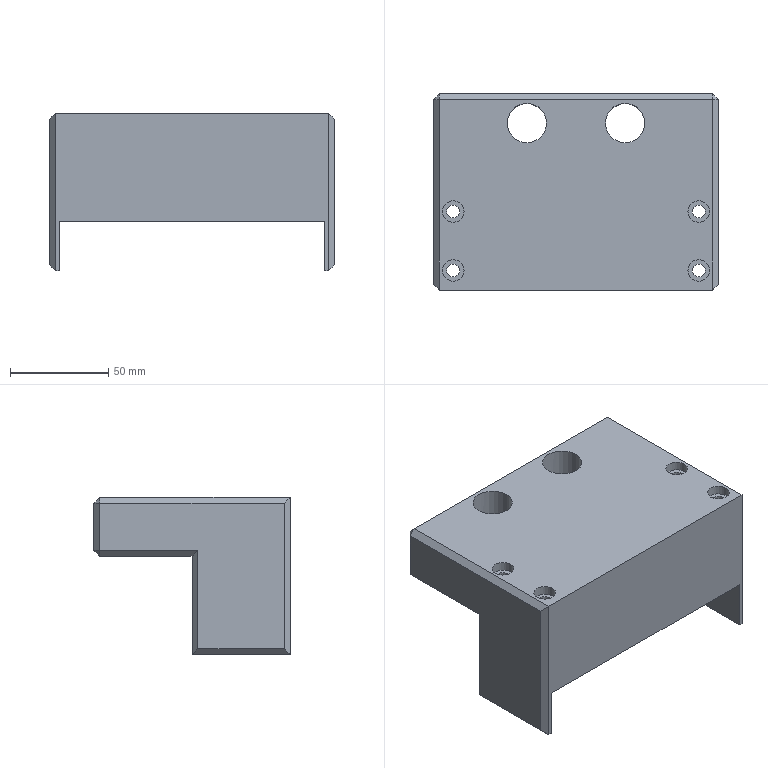NC program | NX | posted with a generic post | part box 145 x 100 x 80 mm
Whole program:
N10 G17 G21 G94 G90
(DRILLING_COPY_2 , TOOL : D8A45)
N12 T06 M6
N14 G54
N16 G17 G0 G90 X-62.5 Y-40. B0. C0. S3000 M3
N18 G43 Z30. H6
N20 G94 G81 G98 Z-1. F150. R3.
N22 Y-10.
N24 X-25. Y35.
N26 X25.
N28 X62.5 Y-10.
N30 Y-40.
N32 G80
N34 G0 X62.5 Y-40. Z30.
N36 M5
(DRILLING_COPY_COPY_COPY_COPY_1_COPY , TOOL : 6.6ZT)
N38 T15 M6
N40 G54
N42 G17 G0 G90 X-62.5 Y-10. B0. C0. S2000 M3
N44 G43 Z30. H15
N46 G94 G83 G98 Z-58.483 F150. Q2. R3.
N48 Y-40.
N50 X62.5
N52 Y-10.
N54 G80
N56 G0 X62.5 Y-10. Z30.
N58 M5
(DRILLING_COPY_COPY_COPY_COPY_1_COPY_COPY , TOOL : 10.5ZT)
N60 T17 M6
N62 G54
N64 G17 G0 G90 X-25. Y35. B0. C0. S1000 M3
N66 G43 Z30. H17
N68 G94 G83 G98 Z-34.655 F150. Q2. R3.
N70 X25.
N72 G80
N74 G0 X25. Y35. Z30.
N76 M5
(刀补12_COPY , TOOL : D10JING)
N78 T04 M6
N80 G54
N82 G17 G0 G90 X-25. Y35. B0. C0. S7000 M3
N84 G43 Z30. H4
N86 Z0.5
N88 G94 G3 X-22.55 Y32.55 R2.45 F1200.
N90 X-20.1 Y35. R2.45
N92 X-20.1 Y35. Z-0.5 I-4.9 J0.
N94 X-20.1 Y35. Z-1.5 I-4.9 J0.
N96 X-20.1 Y35. Z-2.5 I-4.9 J0.
N98 X-20.1 Y35. Z-3.5 I-4.9 J0.
N100 X-20.1 Y35. Z-4.5 I-4.9 J0.
N102 X-20.1 Y35. Z-5.5 I-4.9 J0.
N104 X-20.1 Y35. Z-6.5 I-4.9 J0.
N106 X-20.1 Y35. Z-7.5 I-4.9 J0.
N108 X-20.1 Y35. Z-8.5 I-4.9 J0.
N110 X-20.1 Y35. Z-9.5 I-4.9 J0.
N112 X-20.1 Y35. Z-10.5 I-4.9 J0.
N114 X-20.1 Y35. Z-11.5 I-4.9 J0.
N116 X-20.1 Y35. Z-12.5 I-4.9 J0.
N118 X-20.1 Y35. Z-13.5 I-4.9 J0.
N120 X-20.1 Y35. Z-14.5 I-4.9 J0.
N122 X-20.1 Y35. Z-15.5 I-4.9 J0.
N124 X-20.1 Y35. Z-16.5 I-4.9 J0.
N126 X-20.1 Y35. Z-17.5 I-4.9 J0.
N128 X-20.1 Y35. Z-18.5 I-4.9 J0.
N130 X-20.1 Y35. Z-19.5 I-4.9 J0.
N132 X-20.1 Y35. Z-20.5 I-4.9 J0.
N134 X-20.1 Y35. Z-21.5 I-4.9 J0.
N136 X-20.1 Y35. Z-22.5 I-4.9 J0.
N138 X-20.1 Y35. Z-23.5 I-4.9 J0.
N140 X-20.1 Y35. Z-24.5 I-4.9 J0.
N142 X-20.1 Y35. Z-25.5 I-4.9 J0.
N144 X-20.1 Y35. Z-26.5 I-4.9 J0.
N146 X-20.1 Y35. Z-27.5 I-4.9 J0.
N148 X-20.1 Y35. Z-28.5 I-4.9 J0.
N150 X-20.1 Y35. Z-29.5 I-4.9 J0.
N152 X-29.9 Y35. Z-30. I-4.9 J0.
N154 X-25. Y30.1 R4.9
N156 X-29.9 Y35. R-4.9
N158 X-27.45 Y32.55 R2.45
N160 X-25. Y35. R2.45
N162 G0 Z30.
N164 X25.
N166 Z0.5
N168 G3 X27.45 Y32.55 R2.45
N170 X29.9 Y35. R2.45
N172 X29.9 Y35. Z-0.5 I-4.9 J0.
N174 X29.9 Y35. Z-1.5 I-4.9 J0.
N176 X29.9 Y35. Z-2.5 I-4.9 J0.
N178 X29.9 Y35. Z-3.5 I-4.9 J0.
N180 X29.9 Y35. Z-4.5 I-4.9 J0.
N182 X29.9 Y35. Z-5.5 I-4.9 J0.
N184 X29.9 Y35. Z-6.5 I-4.9 J0.
N186 X29.9 Y35. Z-7.5 I-4.9 J0.
N188 X29.9 Y35. Z-8.5 I-4.9 J0.
N190 X29.9 Y35. Z-9.5 I-4.9 J0.
N192 X29.9 Y35. Z-10.5 I-4.9 J0.
N194 X29.9 Y35. Z-11.5 I-4.9 J0.
N196 X29.9 Y35. Z-12.5 I-4.9 J0.
N198 X29.9 Y35. Z-13.5 I-4.9 J0.
N200 X29.9 Y35. Z-14.5 I-4.9 J0.
N202 X29.9 Y35. Z-15.5 I-4.9 J0.
N204 X29.9 Y35. Z-16.5 I-4.9 J0.
N206 X29.9 Y35. Z-17.5 I-4.9 J0.
N208 X29.9 Y35. Z-18.5 I-4.9 J0.
N210 X29.9 Y35. Z-19.5 I-4.9 J0.
N212 X29.9 Y35. Z-20.5 I-4.9 J0.
N214 X29.9 Y35. Z-21.5 I-4.9 J0.
N216 X29.9 Y35. Z-22.5 I-4.9 J0.
N218 X29.9 Y35. Z-23.5 I-4.9 J0.
N220 X29.9 Y35. Z-24.5 I-4.9 J0.
N222 X29.9 Y35. Z-25.5 I-4.9 J0.
N224 X29.9 Y35. Z-26.5 I-4.9 J0.
N226 X29.9 Y35. Z-27.5 I-4.9 J0.
N228 X29.9 Y35. Z-28.5 I-4.9 J0.
N230 X29.9 Y35. Z-29.5 I-4.9 J0.
N232 X20.1 Y35. Z-30. I-4.9 J0.
N234 X25. Y30.1 R4.9
N236 X20.1 Y35. R-4.9
N238 X22.55 Y32.55 R2.45
N240 X25. Y35. R2.45
N242 G0 Z30.
N244 M5
(HOLE_MILLING , TOOL : D6)
N246 T02 M6
N248 G54
N250 G17 G0 G90 X-62.5 Y-10. B0. C0. S8000 M3
N252 G43 Z30. H2
N254 Z0.5
N256 G94 G3 X-61.25 Y-11.25 R1.25 F1000.
N258 X-60. Y-10. R1.25
N260 X-60. Y-10. Z0. I-2.5 J0.
N262 X-60. Y-10. Z-0.5 I-2.5 J0.
N264 X-60. Y-10. Z-1. I-2.5 J0.
N266 X-60. Y-10. Z-1.5 I-2.5 J0.
N268 X-60. Y-10. Z-2. I-2.5 J0.
N270 X-60. Y-10. Z-2.5 I-2.5 J0.
N272 X-60. Y-10. Z-3. I-2.5 J0.
N274 X-60. Y-10. Z-3.5 I-2.5 J0.
N276 X-60. Y-10. Z-4. I-2.5 J0.
N278 X-60. Y-10. Z-4.5 I-2.5 J0.
N280 X-64.523 Y-8.531 Z-4.7 R2.5
N282 X-63.969 Y-12.023 R2.5
N284 X-64.523 Y-8.531 R-2.5
N286 X-64.246 Y-10.277 R1.25
N288 X-62.5 Y-10. R1.25
N290 G0 Z30.
N292 Y-40.
N294 Z0.5
N296 G3 X-61.25 Y-41.25 R1.25
N298 X-60. Y-40. R1.25
N300 X-60. Y-40. Z0. I-2.5 J0.
N302 X-60. Y-40. Z-0.5 I-2.5 J0.
N304 X-60. Y-40. Z-1. I-2.5 J0.
N306 X-60. Y-40. Z-1.5 I-2.5 J0.
N308 X-60. Y-40. Z-2. I-2.5 J0.
N310 X-60. Y-40. Z-2.5 I-2.5 J0.
N312 X-60. Y-40. Z-3. I-2.5 J0.
N314 X-60. Y-40. Z-3.5 I-2.5 J0.
N316 X-60. Y-40. Z-4. I-2.5 J0.
N318 X-60. Y-40. Z-4.5 I-2.5 J0.
N320 X-64.523 Y-38.531 Z-4.7 R2.5
N322 X-63.969 Y-42.023 R2.5
N324 X-64.523 Y-38.531 R-2.5
N326 X-64.246 Y-40.277 R1.25
N328 X-62.5 Y-40. R1.25
N330 G0 Z30.
N332 X62.5 Y-10.
N334 Z0.5
N336 G3 X63.75 Y-11.25 R1.25
N338 X65. Y-10. R1.25
N340 X65. Y-10. Z0. I-2.5 J0.
N342 X65. Y-10. Z-0.5 I-2.5 J0.
N344 X65. Y-10. Z-1. I-2.5 J0.
N346 X65. Y-10. Z-1.5 I-2.5 J0.
N348 X65. Y-10. Z-2. I-2.5 J0.
N350 X65. Y-10. Z-2.5 I-2.5 J0.
N352 X65. Y-10. Z-3. I-2.5 J0.
N354 X65. Y-10. Z-3.5 I-2.5 J0.
N356 X65. Y-10. Z-4. I-2.5 J0.
N358 X65. Y-10. Z-4.5 I-2.5 J0.
N360 X60.477 Y-8.531 Z-4.7 R2.5
N362 X61.031 Y-12.023 R2.5
N364 X60.477 Y-8.531 R-2.5
N366 X60.754 Y-10.277 R1.25
N368 X62.5 Y-10. R1.25
N370 G0 Z30.
N372 Y-40.
N374 Z0.5
N376 G3 X63.75 Y-41.25 R1.25
N378 X65. Y-40. R1.25
N380 X65. Y-40. Z0. I-2.5 J0.
N382 X65. Y-40. Z-0.5 I-2.5 J0.
N384 X65. Y-40. Z-1. I-2.5 J0.
N386 X65. Y-40. Z-1.5 I-2.5 J0.
N388 X65. Y-40. Z-2. I-2.5 J0.
N390 X65. Y-40. Z-2.5 I-2.5 J0.
N392 X65. Y-40. Z-3. I-2.5 J0.
N394 X65. Y-40. Z-3.5 I-2.5 J0.
N396 X65. Y-40. Z-4. I-2.5 J0.
N398 X65. Y-40. Z-4.5 I-2.5 J0.
N400 X60.477 Y-38.531 Z-4.7 R2.5
N402 X61.031 Y-42.023 R2.5
N404 X60.477 Y-38.531 R-2.5
N406 X60.754 Y-40.277 R1.25
N408 X62.5 Y-40. R1.25
N410 G0 Z30.
N412 M5
(ZLEVEL_PROFILE_1_COPY_1_COPY_COPY_1_COPY_COPY , TOOL : D8A45)
N414 T06 M6
N416 G54
N418 G17 G0 G90 X64.903 Y-11.697 B0. C0. S7500 M3
N420 G43 Z30. H6
N422 Z0.
N424 G94 G1 Z-1. F1000.
N426 X66.641 Y-10.693
N428 G3 X67.041 Y-10. R0.8
N430 X62.5 Y-5.459 R4.541
N432 X67.041 Y-10. R-4.541
N434 X66.641 Y-9.307 R0.8
N436 G1 X64.903 Y-8.303
N438 Z0.
N440 G0 Z30.
N442 X-64.903
N444 Z0.
N446 G1 Z-1.
N448 X-66.641 Y-9.307
N450 G3 X-67.041 Y-10. R0.8
N452 X-62.5 Y-14.541 R4.541
N454 X-67.041 Y-10. R-4.541
N456 X-66.641 Y-10.693 R0.8
N458 G1 X-64.903 Y-11.697
N460 Z0.
N462 G0 Z30.
N464 X60.803 Y-42.403
N466 Z0.
N468 G1 Z-1.
N470 X61.807 Y-44.141
N472 G3 X62.5 Y-44.541 R0.8
N474 X67.041 Y-40. R4.541
N476 X62.5 Y-44.541 R-4.541
N478 X63.193 Y-44.141 R0.8
N480 G1 X64.197 Y-42.403
N482 Z0.
N484 G0 Z30.
N486 X-64.197
N488 Z0.
N490 G1 Z-1.
N492 X-63.193 Y-44.141
N494 G3 X-62.5 Y-44.541 R0.8
N496 X-57.959 Y-40. R4.541
N498 X-62.5 Y-44.541 R-4.541
N500 X-61.807 Y-44.141 R0.8
N502 G1 X-60.803 Y-42.403
N504 Z0.
N506 G0 Z30.
N508 X-23.53 Y42.295
N510 Z0.
N512 G1 Z-1.
N514 X-24.307 Y43.641
N516 G3 X-25. Y44.041 R0.8
N518 X-34.041 Y35. R9.041
N520 X-25. Y44.041 R-9.041
N522 X-25.693 Y43.641 R0.8
N524 G1 X-26.47 Y42.295
N526 Z0.
N528 G0 Z30.
N530 X26.47
N532 Z0.
N534 G1 Z-1.
N536 X25.693 Y43.641
N538 G3 X25. Y44.041 R0.8
N540 X15.959 Y35. R9.041
N542 X25. Y44.041 R-9.041
N544 X24.307 Y43.641 R0.8
N546 G1 X23.53 Y42.295
N548 Z0.
N550 G0 Z30.
(ZLEVEL_PROFILE_1_COPY_1_COPY_COPY_1_COPY_COPY_COPY , TOOL : D8A45)
N552 X70.79 Y-54.933
N554 Z-2.5
N556 G1 Z-3.5
N558 X70.194 Y-53.9
N560 G3 X69.501 Y-53.5 R0.8
N562 G1 X-69.501
N564 G2 X-73. Y-50.017 R3.504
N566 G1 Y-47.001
N568 Y47.001
N570 G2 X-69.504 Y50.5 R3.504
N572 G1 X69.504
N574 G2 X73. Y47.001 R3.504
N576 G1 Y-47.001
N578 Y-50.017
N580 G2 X69.501 Y-53.5 R3.504
N582 G3 X68.809 Y-53.901 R0.8
N584 G1 X68.119 Y-55.1
N586 Z-2.5
N588 G0 Z30.
N590 M5
(刀补12 , TOOL : D10JING)
N592 T04 M6
N594 G54
N596 G17 G0 G90 X-25. Y35. B0. C0. S8000 M3
N598 G43 Z30. H4
N600 Z0.5
N602 G41 G94 G1 X-23.947 Y33.419 F1000. D4
N604 G3 X-20. Y35. R2.29
N606 X-20. Y35. Z-3.5 I-5. J0.
N608 X-20. Y35. Z-7.5 I-5. J0.
N610 X-20. Y35. Z-11.5 I-5. J0.
N612 X-20. Y35. Z-15.5 I-5. J0.
N614 X-20. Y35. Z-19.5 I-5. J0.
N616 X-20. Y35. Z-23.5 I-5. J0.
N618 X-20. Y35. Z-27.5 I-5. J0.
N620 X-28.536 Y31.464 Z-30. R-5.
N622 X-21.464 Y31.464 R5.
N624 X-28.536 Y31.464 R-5.
N626 X-24.627 Y33.137 R2.29
N628 G40
N630 G1 X-25. Y35.
N632 G0 Z30.
N634 X25.
N636 Z0.5
N638 G41 G1 X26.053 Y33.419
N640 G3 X30. Y35. R2.29
N642 X30. Y35. Z-3.5 I-5. J0.
N644 X30. Y35. Z-7.5 I-5. J0.
N646 X30. Y35. Z-11.5 I-5. J0.
N648 X30. Y35. Z-15.5 I-5. J0.
N650 X30. Y35. Z-19.5 I-5. J0.
N652 X30. Y35. Z-23.5 I-5. J0.
N654 X30. Y35. Z-27.5 I-5. J0.
N656 X21.464 Y31.464 Z-30. R-5.
N658 X28.536 Y31.464 R5.
N660 X21.464 Y31.464 R-5.
N662 X25.373 Y33.137 R2.29
N664 G40
N666 G1 X25. Y35.
N668 G0 Z30.
N670 M5
N672 M2